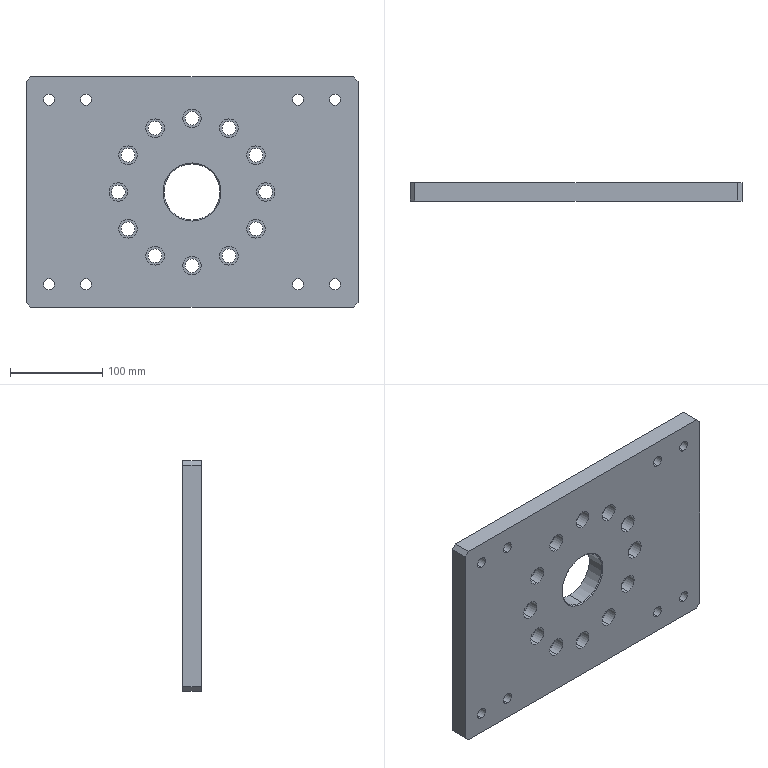Part | SolidWorks | features HoleWzd 3, Chamfer 2, Extrusion 1 | 1 solid | 114 faces | box 360 x 20 x 250 mm | volume 1647177 mm3 | cylinder 82 | plane 30 | cone 2 | commonest cylinder face diameters 15 x24 20 x24 12 x16 18 x16 61 x2